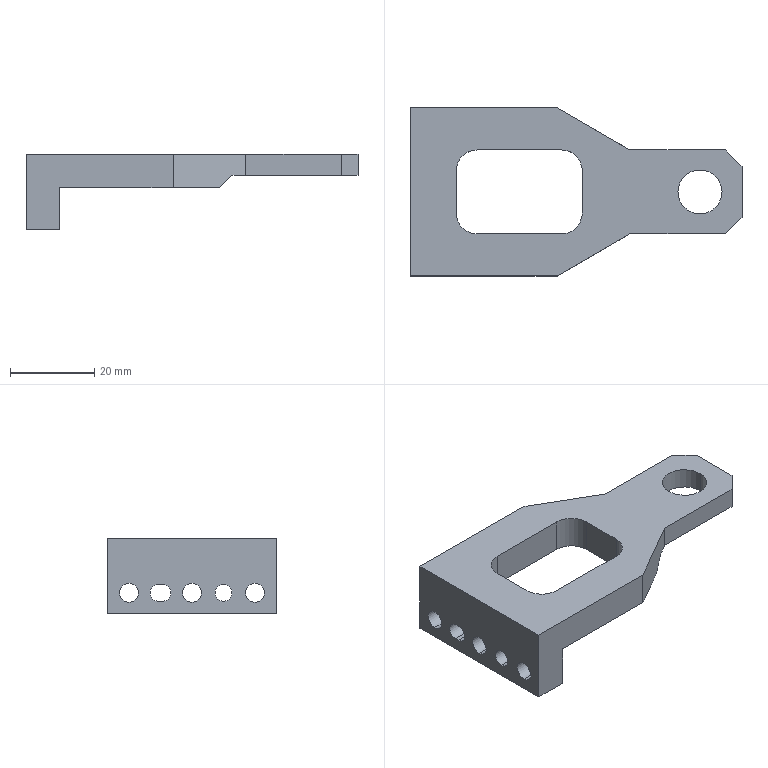Part | SolidWorks | features ICE 6, Chamfer 2, Extrusion 1, HoleWzd 1 | 1 solid | 38 faces | box 79 x 40 x 18 mm | volume 15138 mm3 | plane 22 | cylinder 16 | commonest cylinder face diameters 4.5 x6 4 x4 10 x4 10.5 x2
STEP:
#1=CARTESIAN_POINT('',(8.,12.5,5.601));
#2=VERTEX_POINT('',#1);
#3=CARTESIAN_POINT('',(8.,12.5,9.601));
#4=VERTEX_POINT('',#3);
#5=CARTESIAN_POINT('',(8.,12.5,7.601));
#6=DIRECTION('',(-1.,0.,0.));
#7=DIRECTION('',(0.,0.,1.));
#8=AXIS2_PLACEMENT_3D('',#5,#6,#7);
#9=CIRCLE('',#8,2.);
#10=EDGE_CURVE('',#2,#4,#9,.T.);
#11=ORIENTED_EDGE('',*,*,#10,.F.);
#12=CARTESIAN_POINT('',(0.,12.5,5.601));
#13=VERTEX_POINT('',#12);
#14=CARTESIAN_POINT('',(0.,12.5,5.601));
#15=DIRECTION('',(-1.,0.,0.));
#16=VECTOR('',#15,1000.);
#17=LINE('',#14,#16);
#18=EDGE_CURVE('',#2,#13,#17,.T.);
#19=ORIENTED_EDGE('',*,*,#18,.T.);
#20=CARTESIAN_POINT('',(0.,12.5,9.601));
#21=VERTEX_POINT('',#20);
#22=CARTESIAN_POINT('',(0.,12.5,7.601));
#23=DIRECTION('',(-1.,0.,0.));
#24=DIRECTION('',(0.,0.,1.));
#25=AXIS2_PLACEMENT_3D('',#22,#23,#24);
#26=CIRCLE('',#25,2.);
#27=EDGE_CURVE('',#13,#21,#26,.T.);
#28=ORIENTED_EDGE('',*,*,#27,.T.);
#29=CARTESIAN_POINT('',(0.,12.5,9.601));
#30=DIRECTION('',(-1.,0.,0.));
#31=VECTOR('',#30,1000.);
#32=LINE('',#29,#31);
#33=EDGE_CURVE('',#4,#21,#32,.T.);
#34=ORIENTED_EDGE('',*,*,#33,.F.);
#35=EDGE_LOOP('',(#11,#19,#28,#34));
#36=FACE_OUTER_BOUND('',#35,.T.);
#37=CARTESIAN_POINT('',(0.,12.5,7.601));
#38=DIRECTION('',(-1.,0.,0.));
#39=DIRECTION('',(0.,0.,1.));
#40=AXIS2_PLACEMENT_3D('',#37,#38,#39);
#41=CYLINDRICAL_SURFACE('',#40,2.);
#42=ADVANCED_FACE('',(#36),#41,.F.);
#43=CARTESIAN_POINT('',(0.,5.,9.851));
#44=VERTEX_POINT('',#43);
#45=CARTESIAN_POINT('',(0.,5.,5.351));
#46=VERTEX_POINT('',#45);
#47=CARTESIAN_POINT('',(0.,5.,7.601));
#48=DIRECTION('',(1.,0.,0.));
#49=DIRECTION('',(0.,0.,1.));
#50=AXIS2_PLACEMENT_3D('',#47,#48,#49);
#51=CIRCLE('',#50,2.25);
#52=EDGE_CURVE('',#44,#46,#51,.T.);
#53=ORIENTED_EDGE('',*,*,#52,.F.);
#54=CARTESIAN_POINT('',(8.,5.,9.851));
#55=VERTEX_POINT('',#54);
#56=CARTESIAN_POINT('',(0.,5.,9.851));
#57=DIRECTION('',(1.,0.,0.));
#58=VECTOR('',#57,1000.);
#59=LINE('',#56,#58);
#60=EDGE_CURVE('',#44,#55,#59,.T.);
#61=ORIENTED_EDGE('',*,*,#60,.T.);
#62=CARTESIAN_POINT('',(8.,5.,5.351));
#63=VERTEX_POINT('',#62);
#64=CARTESIAN_POINT('',(8.,5.,7.601));
#65=DIRECTION('',(1.,0.,0.));
#66=DIRECTION('',(0.,0.,1.));
#67=AXIS2_PLACEMENT_3D('',#64,#65,#66);
#68=CIRCLE('',#67,2.25);
#69=EDGE_CURVE('',#55,#63,#68,.T.);
#70=ORIENTED_EDGE('',*,*,#69,.T.);
#71=CARTESIAN_POINT('',(0.,5.,5.351));
#72=DIRECTION('',(1.,0.,0.));
#73=VECTOR('',#72,1000.);
#74=LINE('',#71,#73);
#75=EDGE_CURVE('',#46,#63,#74,.T.);
#76=ORIENTED_EDGE('',*,*,#75,.F.);
#77=EDGE_LOOP('',(#53,#61,#70,#76));
#78=FACE_OUTER_BOUND('',#77,.T.);
#79=CARTESIAN_POINT('',(0.,5.,7.601));
#80=DIRECTION('',(1.,0.,0.));
#81=DIRECTION('',(0.,0.,-1.));
#82=AXIS2_PLACEMENT_3D('',#79,#80,#81);
#83=CYLINDRICAL_SURFACE('',#82,2.25);
#84=ADVANCED_FACE('',(#78),#83,.F.);
#85=CARTESIAN_POINT('',(0.,20.,9.851));
#86=VERTEX_POINT('',#85);
#87=CARTESIAN_POINT('',(0.,20.,5.351));
#88=VERTEX_POINT('',#87);
#89=CARTESIAN_POINT('',(0.,20.,7.601));
#90=DIRECTION('',(1.,0.,0.));
#91=DIRECTION('',(0.,0.,-1.));
#92=AXIS2_PLACEMENT_3D('',#89,#90,#91);
#93=CIRCLE('',#92,2.25);
#94=EDGE_CURVE('',#86,#88,#93,.T.);
#95=ORIENTED_EDGE('',*,*,#94,.F.);
#96=CARTESIAN_POINT('',(8.,20.,9.851));
#97=VERTEX_POINT('',#96);
#98=CARTESIAN_POINT('',(0.,20.,9.851));
#99=DIRECTION('',(1.,0.,0.));
#100=VECTOR('',#99,1000.);
#101=LINE('',#98,#100);
#102=EDGE_CURVE('',#86,#97,#101,.T.);
#103=ORIENTED_EDGE('',*,*,#102,.T.);
#104=CARTESIAN_POINT('',(8.,20.,5.351));
#105=VERTEX_POINT('',#104);
#106=CARTESIAN_POINT('',(8.,20.,7.601));
#107=DIRECTION('',(1.,0.,0.));
#108=DIRECTION('',(0.,0.,-1.));
#109=AXIS2_PLACEMENT_3D('',#106,#107,#108);
#110=CIRCLE('',#109,2.25);
#111=EDGE_CURVE('',#97,#105,#110,.T.);
#112=ORIENTED_EDGE('',*,*,#111,.T.);
#113=CARTESIAN_POINT('',(0.,20.,5.351));
#114=DIRECTION('',(1.,0.,0.));
#115=VECTOR('',#114,1000.);
#116=LINE('',#113,#115);
#117=EDGE_CURVE('',#88,#105,#116,.T.);
#118=ORIENTED_EDGE('',*,*,#117,.F.);
#119=EDGE_LOOP('',(#95,#103,#112,#118));
#120=FACE_OUTER_BOUND('',#119,.T.);
#121=CARTESIAN_POINT('',(0.,20.,7.601));
#122=DIRECTION('',(1.,0.,0.));
#123=DIRECTION('',(0.,0.,-1.));
#124=AXIS2_PLACEMENT_3D('',#121,#122,#123);
#125=CYLINDRICAL_SURFACE('',#124,2.25);
#126=ADVANCED_FACE('',(#120),#125,.F.);
#127=CARTESIAN_POINT('',(0.,35.,9.851));
#128=VERTEX_POINT('',#127);
#129=CARTESIAN_POINT('',(0.,35.,5.351));
#130=VERTEX_POINT('',#129);
#131=CARTESIAN_POINT('',(0.,35.,7.601));
#132=DIRECTION('',(1.,0.,0.));
#133=DIRECTION('',(0.,0.,-1.));
#134=AXIS2_PLACEMENT_3D('',#131,#132,#133);
#135=CIRCLE('',#134,2.25);
#136=EDGE_CURVE('',#128,#130,#135,.T.);
#137=ORIENTED_EDGE('',*,*,#136,.F.);
#138=CARTESIAN_POINT('',(8.,35.,9.851));
#139=VERTEX_POINT('',#138);
#140=CARTESIAN_POINT('',(0.,35.,9.851));
#141=DIRECTION('',(1.,0.,0.));
#142=VECTOR('',#141,1000.);
#143=LINE('',#140,#142);
#144=EDGE_CURVE('',#128,#139,#143,.T.);
#145=ORIENTED_EDGE('',*,*,#144,.T.);
#146=CARTESIAN_POINT('',(8.,35.,5.351));
#147=VERTEX_POINT('',#146);
#148=CARTESIAN_POINT('',(8.,35.,7.601));
#149=DIRECTION('',(1.,0.,0.));
#150=DIRECTION('',(0.,0.,-1.));
#151=AXIS2_PLACEMENT_3D('',#148,#149,#150);
#152=CIRCLE('',#151,2.25);
#153=EDGE_CURVE('',#139,#147,#152,.T.);
#154=ORIENTED_EDGE('',*,*,#153,.T.);
#155=CARTESIAN_POINT('',(0.,35.,5.351));
#156=DIRECTION('',(1.,0.,0.));
#157=VECTOR('',#156,1000.);
#158=LINE('',#155,#157);
#159=EDGE_CURVE('',#130,#147,#158,.T.);
#160=ORIENTED_EDGE('',*,*,#159,.F.);
#161=EDGE_LOOP('',(#137,#145,#154,#160));
#162=FACE_OUTER_BOUND('',#161,.T.);
#163=CARTESIAN_POINT('',(0.,35.,7.601));
#164=DIRECTION('',(1.,0.,0.));
#165=DIRECTION('',(0.,0.,-1.));
#166=AXIS2_PLACEMENT_3D('',#163,#164,#165);
#167=CYLINDRICAL_SURFACE('',#166,2.25);
#168=ADVANCED_FACE('',(#162),#167,.F.);
#169=CARTESIAN_POINT('',(74.25,20.,20.601));
#170=VERTEX_POINT('',#169);
#171=CARTESIAN_POINT('',(63.75,20.,20.601));
#172=VERTEX_POINT('',#171);
#173=CARTESIAN_POINT('',(69.,20.,20.601));
#174=DIRECTION('',(0.,0.,-1.));
#175=DIRECTION('',(-1.,0.,0.));
#176=AXIS2_PLACEMENT_3D('',#173,#174,#175);
#177=CIRCLE('',#176,5.25);
#178=EDGE_CURVE('',#170,#172,#177,.T.);
#179=ORIENTED_EDGE('',*,*,#178,.F.);
#180=CARTESIAN_POINT('',(74.25,20.,15.601));
#181=VERTEX_POINT('',#180);
#182=CARTESIAN_POINT('',(74.25,20.,22.601));
#183=DIRECTION('',(0.,0.,-1.));
#184=VECTOR('',#183,1000.);
#185=LINE('',#182,#184);
#186=EDGE_CURVE('',#170,#181,#185,.T.);
#187=ORIENTED_EDGE('',*,*,#186,.T.);
#188=CARTESIAN_POINT('',(63.75,20.,15.601));
#189=VERTEX_POINT('',#188);
#190=CARTESIAN_POINT('',(69.,20.,15.601));
#191=DIRECTION('',(0.,0.,-1.));
#192=DIRECTION('',(1.,0.,0.));
#193=AXIS2_PLACEMENT_3D('',#190,#191,#192);
#194=CIRCLE('',#193,5.25);
#195=EDGE_CURVE('',#181,#189,#194,.T.);
#196=ORIENTED_EDGE('',*,*,#195,.T.);
#197=CARTESIAN_POINT('',(63.75,20.,22.601));
#198=DIRECTION('',(0.,0.,-1.));
#199=VECTOR('',#198,1000.);
#200=LINE('',#197,#199);
#201=EDGE_CURVE('',#172,#189,#200,.T.);
#202=ORIENTED_EDGE('',*,*,#201,.F.);
#203=EDGE_LOOP('',(#179,#187,#196,#202));
#204=FACE_OUTER_BOUND('',#203,.T.);
#205=CARTESIAN_POINT('',(69.,20.,22.601));
#206=DIRECTION('',(0.,0.,-1.));
#207=DIRECTION('',(-1.,0.,0.));
#208=AXIS2_PLACEMENT_3D('',#205,#206,#207);
#209=CYLINDRICAL_SURFACE('',#208,5.25);
#210=ADVANCED_FACE('',(#204),#209,.F.);
#211=CARTESIAN_POINT('',(8.,27.,9.601));
#212=VERTEX_POINT('',#211);
#213=CARTESIAN_POINT('',(8.,28.,9.601));
#214=VERTEX_POINT('',#213);
#215=CARTESIAN_POINT('',(8.,40.,9.601));
#216=DIRECTION('',(0.,1.,0.));
#217=VECTOR('',#216,1000.);
#218=LINE('',#215,#217);
#219=EDGE_CURVE('',#212,#214,#218,.T.);
#220=ORIENTED_EDGE('',*,*,#219,.T.);
#221=CARTESIAN_POINT('',(8.,28.,5.601));
#222=VERTEX_POINT('',#221);
#223=CARTESIAN_POINT('',(8.,28.,7.601));
#224=DIRECTION('',(-1.,0.,0.));
#225=DIRECTION('',(0.,0.,1.));
#226=AXIS2_PLACEMENT_3D('',#223,#224,#225);
#227=CIRCLE('',#226,2.);
#228=EDGE_CURVE('',#214,#222,#227,.T.);
#229=ORIENTED_EDGE('',*,*,#228,.T.);
#230=CARTESIAN_POINT('',(8.,27.,5.601));
#231=VERTEX_POINT('',#230);
#232=CARTESIAN_POINT('',(8.,40.,5.601));
#233=DIRECTION('',(0.,-1.,0.));
#234=VECTOR('',#233,1000.);
#235=LINE('',#232,#234);
#236=EDGE_CURVE('',#222,#231,#235,.T.);
#237=ORIENTED_EDGE('',*,*,#236,.T.);
#238=CARTESIAN_POINT('',(8.,27.,7.601));
#239=DIRECTION('',(-1.,0.,0.));
#240=DIRECTION('',(0.,0.,1.));
#241=AXIS2_PLACEMENT_3D('',#238,#239,#240);
#242=CIRCLE('',#241,2.);
#243=EDGE_CURVE('',#231,#212,#242,.T.);
#244=ORIENTED_EDGE('',*,*,#243,.T.);
#245=EDGE_LOOP('',(#220,#229,#237,#244));
#246=FACE_BOUND('',#245,.T.);
#247=CARTESIAN_POINT('',(8.,12.5,7.601));
#248=DIRECTION('',(-1.,0.,0.));
#249=DIRECTION('',(0.,0.,1.));
#250=AXIS2_PLACEMENT_3D('',#247,#248,#249);
#251=CIRCLE('',#250,2.);
#252=EDGE_CURVE('',#4,#2,#251,.T.);
#253=ORIENTED_EDGE('',*,*,#252,.T.);
#254=ORIENTED_EDGE('',*,*,#10,.T.);
#255=EDGE_LOOP('',(#253,#254));
#256=FACE_BOUND('',#255,.T.);
#257=CARTESIAN_POINT('',(8.,5.,7.601));
#258=DIRECTION('',(1.,0.,0.));
#259=DIRECTION('',(0.,0.,1.));
#260=AXIS2_PLACEMENT_3D('',#257,#258,#259);
#261=CIRCLE('',#260,2.25);
#262=EDGE_CURVE('',#63,#55,#261,.T.);
#263=ORIENTED_EDGE('',*,*,#262,.F.);
#264=ORIENTED_EDGE('',*,*,#69,.F.);
#265=EDGE_LOOP('',(#263,#264));
#266=FACE_BOUND('',#265,.T.);
#267=CARTESIAN_POINT('',(8.,20.,7.601));
#268=DIRECTION('',(1.,0.,0.));
#269=DIRECTION('',(0.,0.,-1.));
#270=AXIS2_PLACEMENT_3D('',#267,#268,#269);
#271=CIRCLE('',#270,2.25);
#272=EDGE_CURVE('',#105,#97,#271,.T.);
#273=ORIENTED_EDGE('',*,*,#272,.F.);
#274=ORIENTED_EDGE('',*,*,#111,.F.);
#275=EDGE_LOOP('',(#273,#274));
#276=FACE_BOUND('',#275,.T.);
#277=CARTESIAN_POINT('',(8.,35.,7.601));
#278=DIRECTION('',(1.,0.,0.));
#279=DIRECTION('',(0.,0.,-1.));
#280=AXIS2_PLACEMENT_3D('',#277,#278,#279);
#281=CIRCLE('',#280,2.25);
#282=EDGE_CURVE('',#147,#139,#281,.T.);
#283=ORIENTED_EDGE('',*,*,#282,.F.);
#284=ORIENTED_EDGE('',*,*,#153,.F.);
#285=EDGE_LOOP('',(#283,#284));
#286=FACE_BOUND('',#285,.T.);
#287=CARTESIAN_POINT('',(8.,0.,12.601));
#288=VERTEX_POINT('',#287);
#289=CARTESIAN_POINT('',(8.,0.,2.601));
#290=VERTEX_POINT('',#289);
#291=CARTESIAN_POINT('',(8.,0.,12.601));
#292=DIRECTION('',(0.,0.,-1.));
#293=VECTOR('',#292,1000.);
#294=LINE('',#291,#293);
#295=EDGE_CURVE('',#288,#290,#294,.T.);
#296=ORIENTED_EDGE('',*,*,#295,.T.);
#297=CARTESIAN_POINT('',(8.,40.,2.601));
#298=VERTEX_POINT('',#297);
#299=CARTESIAN_POINT('',(8.,40.,2.601));
#300=DIRECTION('',(0.,-1.,0.));
#301=VECTOR('',#300,1000.);
#302=LINE('',#299,#301);
#303=EDGE_CURVE('',#298,#290,#302,.T.);
#304=ORIENTED_EDGE('',*,*,#303,.F.);
#305=CARTESIAN_POINT('',(8.,40.,12.601));
#306=VERTEX_POINT('',#305);
#307=CARTESIAN_POINT('',(8.,40.,12.601));
#308=DIRECTION('',(0.,0.,-1.));
#309=VECTOR('',#308,1000.);
#310=LINE('',#307,#309);
#311=EDGE_CURVE('',#306,#298,#310,.T.);
#312=ORIENTED_EDGE('',*,*,#311,.F.);
#313=CARTESIAN_POINT('',(8.,40.,12.601));
#314=DIRECTION('',(0.,-1.,0.));
#315=VECTOR('',#314,1000.);
#316=LINE('',#313,#315);
#317=EDGE_CURVE('',#306,#288,#316,.T.);
#318=ORIENTED_EDGE('',*,*,#317,.T.);
#319=EDGE_LOOP('',(#296,#304,#312,#318));
#320=FACE_OUTER_BOUND('',#319,.T.);
#321=CARTESIAN_POINT('',(8.,40.,12.601));
#322=DIRECTION('',(-1.,0.,0.));
#323=DIRECTION('',(0.,0.,1.));
#324=AXIS2_PLACEMENT_3D('',#321,#322,#323);
#325=PLANE('',#324);
#326=ADVANCED_FACE('',(#246,#256,#266,#276,#286,#320),#325,.F.);
#327=CARTESIAN_POINT('',(0.,0.,2.601));
#328=VERTEX_POINT('',#327);
#329=CARTESIAN_POINT('',(0.,0.,2.601));
#330=DIRECTION('',(-1.,0.,0.));
#331=VECTOR('',#330,1000.);
#332=LINE('',#329,#331);
#333=EDGE_CURVE('',#290,#328,#332,.T.);
#334=ORIENTED_EDGE('',*,*,#333,.T.);
#335=CARTESIAN_POINT('',(0.,40.,2.601));
#336=VERTEX_POINT('',#335);
#337=CARTESIAN_POINT('',(0.,40.,2.601));
#338=DIRECTION('',(0.,-1.,0.));
#339=VECTOR('',#338,1000.);
#340=LINE('',#337,#339);
#341=EDGE_CURVE('',#336,#328,#340,.T.);
#342=ORIENTED_EDGE('',*,*,#341,.F.);
#343=CARTESIAN_POINT('',(0.,40.,2.601));
#344=DIRECTION('',(-1.,0.,0.));
#345=VECTOR('',#344,1000.);
#346=LINE('',#343,#345);
#347=EDGE_CURVE('',#298,#336,#346,.T.);
#348=ORIENTED_EDGE('',*,*,#347,.F.);
#349=ORIENTED_EDGE('',*,*,#303,.T.);
#350=EDGE_LOOP('',(#334,#342,#348,#349));
#351=FACE_OUTER_BOUND('',#350,.T.);
#352=CARTESIAN_POINT('',(0.,40.,2.601));
#353=DIRECTION('',(0.,0.,1.));
#354=DIRECTION('',(1.,0.,0.));
#355=AXIS2_PLACEMENT_3D('',#352,#353,#354);
#356=PLANE('',#355);
#357=ADVANCED_FACE('',(#351),#356,.F.);
#358=CARTESIAN_POINT('',(0.,28.,5.601));
#359=VERTEX_POINT('',#358);
#360=CARTESIAN_POINT('',(0.,27.,5.601));
#361=VERTEX_POINT('',#360);
#362=CARTESIAN_POINT('',(0.,28.,5.601));
#363=DIRECTION('',(0.,-1.,0.));
#364=VECTOR('',#363,1000.);
#365=LINE('',#362,#364);
#366=EDGE_CURVE('',#359,#361,#365,.T.);
#367=ORIENTED_EDGE('',*,*,#366,.F.);
#368=CARTESIAN_POINT('',(0.,28.,9.601));
#369=VERTEX_POINT('',#368);
#370=CARTESIAN_POINT('',(0.,28.,7.601));
#371=DIRECTION('',(-1.,0.,0.));
#372=DIRECTION('',(0.,0.,1.));
#373=AXIS2_PLACEMENT_3D('',#370,#371,#372);
#374=CIRCLE('',#373,2.);
#375=EDGE_CURVE('',#369,#359,#374,.T.);
#376=ORIENTED_EDGE('',*,*,#375,.F.);
#377=CARTESIAN_POINT('',(0.,27.,9.601));
#378=VERTEX_POINT('',#377);
#379=CARTESIAN_POINT('',(0.,28.,9.601));
#380=DIRECTION('',(0.,1.,0.));
#381=VECTOR('',#380,1000.);
#382=LINE('',#379,#381);
#383=EDGE_CURVE('',#378,#369,#382,.T.);
#384=ORIENTED_EDGE('',*,*,#383,.F.);
#385=CARTESIAN_POINT('',(0.,27.,7.601));
#386=DIRECTION('',(-1.,0.,0.));
#387=DIRECTION('',(0.,0.,1.));
#388=AXIS2_PLACEMENT_3D('',#385,#386,#387);
#389=CIRCLE('',#388,2.);
#390=EDGE_CURVE('',#361,#378,#389,.T.);
#391=ORIENTED_EDGE('',*,*,#390,.F.);
#392=EDGE_LOOP('',(#367,#376,#384,#391));
#393=FACE_BOUND('',#392,.T.);
#394=CARTESIAN_POINT('',(0.,12.5,7.601));
#395=DIRECTION('',(-1.,0.,0.));
#396=DIRECTION('',(0.,0.,1.));
#397=AXIS2_PLACEMENT_3D('',#394,#395,#396);
#398=CIRCLE('',#397,2.);
#399=EDGE_CURVE('',#21,#13,#398,.T.);
#400=ORIENTED_EDGE('',*,*,#399,.F.);
#401=ORIENTED_EDGE('',*,*,#27,.F.);
#402=EDGE_LOOP('',(#400,#401));
#403=FACE_BOUND('',#402,.T.);
#404=CARTESIAN_POINT('',(0.,5.,7.601));
#405=DIRECTION('',(1.,0.,0.));
#406=DIRECTION('',(0.,0.,1.));
#407=AXIS2_PLACEMENT_3D('',#404,#405,#406);
#408=CIRCLE('',#407,2.25);
#409=EDGE_CURVE('',#46,#44,#408,.T.);
#410=ORIENTED_EDGE('',*,*,#409,.T.);
#411=ORIENTED_EDGE('',*,*,#52,.T.);
#412=EDGE_LOOP('',(#410,#411));
#413=FACE_BOUND('',#412,.T.);
#414=CARTESIAN_POINT('',(0.,20.,7.601));
#415=DIRECTION('',(1.,0.,0.));
#416=DIRECTION('',(0.,0.,-1.));
#417=AXIS2_PLACEMENT_3D('',#414,#415,#416);
#418=CIRCLE('',#417,2.25);
#419=EDGE_CURVE('',#88,#86,#418,.T.);
#420=ORIENTED_EDGE('',*,*,#419,.T.);
#421=ORIENTED_EDGE('',*,*,#94,.T.);
#422=EDGE_LOOP('',(#420,#421));
#423=FACE_BOUND('',#422,.T.);
#424=CARTESIAN_POINT('',(0.,35.,7.601));
#425=DIRECTION('',(1.,0.,0.));
#426=DIRECTION('',(0.,0.,-1.));
#427=AXIS2_PLACEMENT_3D('',#424,#425,#426);
#428=CIRCLE('',#427,2.25);
#429=EDGE_CURVE('',#130,#128,#428,.T.);
#430=ORIENTED_EDGE('',*,*,#429,.T.);
#431=ORIENTED_EDGE('',*,*,#136,.T.);
#432=EDGE_LOOP('',(#430,#431));
#433=FACE_BOUND('',#432,.T.);
#434=CARTESIAN_POINT('',(0.,0.,20.601));
#435=VERTEX_POINT('',#434);
#436=CARTESIAN_POINT('',(0.,0.,20.601));
#437=DIRECTION('',(0.,0.,1.));
#438=VECTOR('',#437,1000.);
#439=LINE('',#436,#438);
#440=EDGE_CURVE('',#328,#435,#439,.T.);
#441=ORIENTED_EDGE('',*,*,#440,.T.);
#442=CARTESIAN_POINT('',(0.,40.,20.601));
#443=VERTEX_POINT('',#442);
#444=CARTESIAN_POINT('',(0.,40.,20.601));
#445=DIRECTION('',(0.,-1.,0.));
#446=VECTOR('',#445,1000.);
#447=LINE('',#444,#446);
#448=EDGE_CURVE('',#443,#435,#447,.T.);
#449=ORIENTED_EDGE('',*,*,#448,.F.);
#450=CARTESIAN_POINT('',(0.,40.,20.601));
#451=DIRECTION('',(0.,0.,1.));
#452=VECTOR('',#451,1000.);
#453=LINE('',#450,#452);
#454=EDGE_CURVE('',#336,#443,#453,.T.);
#455=ORIENTED_EDGE('',*,*,#454,.F.);
#456=ORIENTED_EDGE('',*,*,#341,.T.);
#457=EDGE_LOOP('',(#441,#449,#455,#456));
#458=FACE_OUTER_BOUND('',#457,.T.);
#459=CARTESIAN_POINT('',(0.,40.,20.601));
#460=DIRECTION('',(1.,0.,0.));
#461=DIRECTION('',(0.,0.,-1.));
#462=AXIS2_PLACEMENT_3D('',#459,#460,#461);
#463=PLANE('',#462);
#464=ADVANCED_FACE('',(#393,#403,#413,#423,#433,#458),#463,.F.);
#465=CARTESIAN_POINT('',(11.,25.,20.601));
#466=VERTEX_POINT('',#465);
#467=CARTESIAN_POINT('',(11.,15.,20.601));
#468=VERTEX_POINT('',#467);
#469=CARTESIAN_POINT('',(11.,15.,20.601));
#470=DIRECTION('',(0.,-1.,0.));
#471=VECTOR('',#470,1000.);
#472=LINE('',#469,#471);
#473=EDGE_CURVE('',#466,#468,#472,.T.);
#474=ORIENTED_EDGE('',*,*,#473,.F.);
#475=CARTESIAN_POINT('',(16.,30.,20.601));
#476=VERTEX_POINT('',#475);
#477=CARTESIAN_POINT('',(16.,25.,20.601));
#478=DIRECTION('',(0.,0.,1.));
#479=DIRECTION('',(1.,0.,0.));
#480=AXIS2_PLACEMENT_3D('',#477,#478,#479);
#481=CIRCLE('',#480,5.);
#482=EDGE_CURVE('',#476,#466,#481,.T.);
#483=ORIENTED_EDGE('',*,*,#482,.F.);
#484=CARTESIAN_POINT('',(36.,30.,20.601));
#485=VERTEX_POINT('',#484);
#486=CARTESIAN_POINT('',(16.,30.,20.601));
#487=DIRECTION('',(-1.,0.,0.));
#488=VECTOR('',#487,1000.);
#489=LINE('',#486,#488);
#490=EDGE_CURVE('',#485,#476,#489,.T.);
#491=ORIENTED_EDGE('',*,*,#490,.F.);
#492=CARTESIAN_POINT('',(41.,25.,20.601));
#493=VERTEX_POINT('',#492);
#494=CARTESIAN_POINT('',(36.,25.,20.601));
#495=DIRECTION('',(0.,0.,1.));
#496=DIRECTION('',(1.,0.,0.));
#497=AXIS2_PLACEMENT_3D('',#494,#495,#496);
#498=CIRCLE('',#497,5.);
#499=EDGE_CURVE('',#493,#485,#498,.T.);
#500=ORIENTED_EDGE('',*,*,#499,.F.);
#501=CARTESIAN_POINT('',(41.,15.,20.601));
#502=VERTEX_POINT('',#501);
#503=CARTESIAN_POINT('',(41.,15.,20.601));
#504=DIRECTION('',(0.,1.,0.));
#505=VECTOR('',#504,1000.);
#506=LINE('',#503,#505);
#507=EDGE_CURVE('',#502,#493,#506,.T.);
#508=ORIENTED_EDGE('',*,*,#507,.F.);
#509=CARTESIAN_POINT('',(36.,10.,20.601));
#510=VERTEX_POINT('',#509);
#511=CARTESIAN_POINT('',(36.,15.,20.601));
#512=DIRECTION('',(0.,0.,1.));
#513=DIRECTION('',(1.,0.,0.));
#514=AXIS2_PLACEMENT_3D('',#511,#512,#513);
#515=CIRCLE('',#514,5.);
#516=EDGE_CURVE('',#510,#502,#515,.T.);
#517=ORIENTED_EDGE('',*,*,#516,.F.);
#518=CARTESIAN_POINT('',(16.,10.,20.601));
#519=VERTEX_POINT('',#518);
#520=CARTESIAN_POINT('',(16.,10.,20.601));
#521=DIRECTION('',(1.,0.,0.));
#522=VECTOR('',#521,1000.);
#523=LINE('',#520,#522);
#524=EDGE_CURVE('',#519,#510,#523,.T.);
#525=ORIENTED_EDGE('',*,*,#524,.F.);
#526=CARTESIAN_POINT('',(16.,15.,20.601));
#527=DIRECTION('',(0.,0.,1.));
#528=DIRECTION('',(1.,0.,0.));
#529=AXIS2_PLACEMENT_3D('',#526,#527,#528);
#530=CIRCLE('',#529,5.);
#531=EDGE_CURVE('',#468,#519,#530,.T.);
#532=ORIENTED_EDGE('',*,*,#531,.F.);
#533=EDGE_LOOP('',(#474,#483,#491,#500,#508,#517,#525,#532));
#534=FACE_BOUND('',#533,.T.);
#535=CARTESIAN_POINT('',(69.,20.,20.601));
#536=DIRECTION('',(0.,0.,-1.));
#537=DIRECTION('',(-1.,0.,0.));
#538=AXIS2_PLACEMENT_3D('',#535,#536,#537);
#539=CIRCLE('',#538,5.25);
#540=EDGE_CURVE('',#172,#170,#539,.T.);
#541=ORIENTED_EDGE('',*,*,#540,.T.);
#542=ORIENTED_EDGE('',*,*,#178,.T.);
#543=EDGE_LOOP('',(#541,#542));
#544=FACE_BOUND('',#543,.T.);
#545=CARTESIAN_POINT('',(75.,10.,20.601));
#546=VERTEX_POINT('',#545);
#547=CARTESIAN_POINT('',(52.321,10.,20.601));
#548=VERTEX_POINT('',#547);
#549=CARTESIAN_POINT('',(79.,10.,20.601));
#550=DIRECTION('',(-1.,0.,0.));
#551=VECTOR('',#550,1000.);
#552=LINE('',#549,#551);
#553=EDGE_CURVE('',#546,#548,#552,.T.);
#554=ORIENTED_EDGE('',*,*,#553,.F.);
#555=CARTESIAN_POINT('',(79.,14.,20.601));
#556=VERTEX_POINT('',#555);
#557=CARTESIAN_POINT('',(75.,10.,20.601));
#558=DIRECTION('',(0.7071,0.7071,0.));
#559=VECTOR('',#558,1000.);
#560=LINE('',#557,#559);
#561=EDGE_CURVE('',#546,#556,#560,.T.);
#562=ORIENTED_EDGE('',*,*,#561,.T.);
#563=CARTESIAN_POINT('',(79.,26.,20.601));
#564=VERTEX_POINT('',#563);
#565=CARTESIAN_POINT('',(79.,40.,20.601));
#566=DIRECTION('',(0.,-1.,0.));
#567=VECTOR('',#566,1000.);
#568=LINE('',#565,#567);
#569=EDGE_CURVE('',#564,#556,#568,.T.);
#570=ORIENTED_EDGE('',*,*,#569,.F.);
#571=CARTESIAN_POINT('',(75.,30.,20.601));
#572=VERTEX_POINT('',#571);
#573=CARTESIAN_POINT('',(79.,26.,20.601));
#574=DIRECTION('',(-0.7071,0.7071,0.));
#575=VECTOR('',#574,1000.);
#576=LINE('',#573,#575);
#577=EDGE_CURVE('',#564,#572,#576,.T.);
#578=ORIENTED_EDGE('',*,*,#577,.T.);
#579=CARTESIAN_POINT('',(52.321,30.,20.601));
#580=VERTEX_POINT('',#579);
#581=CARTESIAN_POINT('',(79.,30.,20.601));
#582=DIRECTION('',(1.,0.,0.));
#583=VECTOR('',#582,1000.);
#584=LINE('',#581,#583);
#585=EDGE_CURVE('',#580,#572,#584,.T.);
#586=ORIENTED_EDGE('',*,*,#585,.F.);
#587=CARTESIAN_POINT('',(35.,40.,20.601));
#588=VERTEX_POINT('',#587);
#589=CARTESIAN_POINT('',(35.,40.,20.601));
#590=DIRECTION('',(0.866,-0.5,0.));
#591=VECTOR('',#590,1000.);
#592=LINE('',#589,#591);
#593=EDGE_CURVE('',#588,#580,#592,.T.);
#594=ORIENTED_EDGE('',*,*,#593,.F.);
#595=CARTESIAN_POINT('',(0.,40.,20.601));
#596=DIRECTION('',(1.,0.,0.));
#597=VECTOR('',#596,1000.);
#598=LINE('',#595,#597);
#599=EDGE_CURVE('',#443,#588,#598,.T.);
#600=ORIENTED_EDGE('',*,*,#599,.F.);
#601=ORIENTED_EDGE('',*,*,#448,.T.);
#602=CARTESIAN_POINT('',(35.,0.,20.601));
#603=VERTEX_POINT('',#602);
#604=CARTESIAN_POINT('',(0.,0.,20.601));
#605=DIRECTION('',(1.,0.,0.));
#606=VECTOR('',#605,1000.);
#607=LINE('',#604,#606);
#608=EDGE_CURVE('',#435,#603,#607,.T.);
#609=ORIENTED_EDGE('',*,*,#608,.T.);
#610=CARTESIAN_POINT('',(35.,0.,20.601));
#611=DIRECTION('',(-0.866,-0.5,0.));
#612=VECTOR('',#611,1000.);
#613=LINE('',#610,#612);
#614=EDGE_CURVE('',#548,#603,#613,.T.);
#615=ORIENTED_EDGE('',*,*,#614,.F.);
#616=EDGE_LOOP('',(#554,#562,#570,#578,#586,#594,#600,#601,#609,#615));
#617=FACE_OUTER_BOUND('',#616,.T.);
#618=CARTESIAN_POINT('',(0.,40.,20.601));
#619=DIRECTION('',(0.,0.,-1.));
#620=DIRECTION('',(-1.,0.,0.));
#621=AXIS2_PLACEMENT_3D('',#618,#619,#620);
#622=PLANE('',#621);
#623=ADVANCED_FACE('',(#534,#544,#617),#622,.F.);
#624=ORIENTED_EDGE('',*,*,#569,.T.);
#625=CARTESIAN_POINT('',(79.,14.,15.601));
#626=VERTEX_POINT('',#625);
#627=CARTESIAN_POINT('',(79.,14.,20.601));
#628=DIRECTION('',(0.,0.,-1.));
#629=VECTOR('',#628,1000.);
#630=LINE('',#627,#629);
#631=EDGE_CURVE('',#556,#626,#630,.T.);
#632=ORIENTED_EDGE('',*,*,#631,.T.);
#633=CARTESIAN_POINT('',(79.,26.,15.601));
#634=VERTEX_POINT('',#633);
#635=CARTESIAN_POINT('',(79.,0.,15.601));
#636=DIRECTION('',(0.,1.,0.));
#637=VECTOR('',#636,1000.);
#638=LINE('',#635,#637);
#639=EDGE_CURVE('',#626,#634,#638,.T.);
#640=ORIENTED_EDGE('',*,*,#639,.T.);
#641=CARTESIAN_POINT('',(79.,26.,20.601));
#642=DIRECTION('',(0.,0.,1.));
#643=VECTOR('',#642,1000.);
#644=LINE('',#641,#643);
#645=EDGE_CURVE('',#634,#564,#644,.T.);
#646=ORIENTED_EDGE('',*,*,#645,.T.);
#647=EDGE_LOOP('',(#624,#632,#640,#646));
#648=FACE_OUTER_BOUND('',#647,.T.);
#649=CARTESIAN_POINT('',(79.,40.,20.601));
#650=DIRECTION('',(-1.,0.,0.));
#651=DIRECTION('',(0.,0.,1.));
#652=AXIS2_PLACEMENT_3D('',#649,#650,#651);
#653=PLANE('',#652);
#654=ADVANCED_FACE('',(#648),#653,.F.);
#655=CARTESIAN_POINT('',(36.,30.,12.601));
#656=VERTEX_POINT('',#655);
#657=CARTESIAN_POINT('',(16.,30.,12.601));
#658=VERTEX_POINT('',#657);
#659=CARTESIAN_POINT('',(79.,30.,12.601));
#660=DIRECTION('',(-1.,0.,0.));
#661=VECTOR('',#660,1000.);
#662=LINE('',#659,#661);
#663=EDGE_CURVE('',#656,#658,#662,.T.);
#664=ORIENTED_EDGE('',*,*,#663,.T.);
#665=CARTESIAN_POINT('',(11.,25.,12.601));
#666=VERTEX_POINT('',#665);
#667=CARTESIAN_POINT('',(16.,25.,12.601));
#668=DIRECTION('',(0.,0.,1.));
#669=DIRECTION('',(1.,0.,0.));
#670=AXIS2_PLACEMENT_3D('',#667,#668,#669);
#671=CIRCLE('',#670,5.);
#672=EDGE_CURVE('',#658,#666,#671,.T.);
#673=ORIENTED_EDGE('',*,*,#672,.T.);
#674=CARTESIAN_POINT('',(11.,15.,12.601));
#675=VERTEX_POINT('',#674);
#676=CARTESIAN_POINT('',(11.,40.,12.601));
#677=DIRECTION('',(0.,-1.,0.));
#678=VECTOR('',#677,1000.);
#679=LINE('',#676,#678);
#680=EDGE_CURVE('',#666,#675,#679,.T.);
#681=ORIENTED_EDGE('',*,*,#680,.T.);
#682=CARTESIAN_POINT('',(16.,10.,12.601));
#683=VERTEX_POINT('',#682);
#684=CARTESIAN_POINT('',(16.,15.,12.601));
#685=DIRECTION('',(0.,0.,1.));
#686=DIRECTION('',(1.,0.,0.));
#687=AXIS2_PLACEMENT_3D('',#684,#685,#686);
#688=CIRCLE('',#687,5.);
#689=EDGE_CURVE('',#675,#683,#688,.T.);
#690=ORIENTED_EDGE('',*,*,#689,.T.);
#691=CARTESIAN_POINT('',(36.,10.,12.601));
#692=VERTEX_POINT('',#691);
#693=CARTESIAN_POINT('',(79.,10.,12.601));
#694=DIRECTION('',(1.,0.,0.));
#695=VECTOR('',#694,1000.);
#696=LINE('',#693,#695);
#697=EDGE_CURVE('',#683,#692,#696,.T.);
#698=ORIENTED_EDGE('',*,*,#697,.T.);
#699=CARTESIAN_POINT('',(41.,15.,12.601));
#700=VERTEX_POINT('',#699);
#701=CARTESIAN_POINT('',(36.,15.,12.601));
#702=DIRECTION('',(0.,0.,1.));
#703=DIRECTION('',(1.,0.,0.));
#704=AXIS2_PLACEMENT_3D('',#701,#702,#703);
#705=CIRCLE('',#704,5.);
#706=EDGE_CURVE('',#692,#700,#705,.T.);
#707=ORIENTED_EDGE('',*,*,#706,.T.);
#708=CARTESIAN_POINT('',(41.,25.,12.601));
#709=VERTEX_POINT('',#708);
#710=CARTESIAN_POINT('',(41.,40.,12.601));
#711=DIRECTION('',(0.,1.,0.));
#712=VECTOR('',#711,1000.);
#713=LINE('',#710,#712);
#714=EDGE_CURVE('',#700,#709,#713,.T.);
#715=ORIENTED_EDGE('',*,*,#714,.T.);
#716=CARTESIAN_POINT('',(36.,25.,12.601));
#717=DIRECTION('',(0.,0.,1.));
#718=DIRECTION('',(1.,0.,0.));
#719=AXIS2_PLACEMENT_3D('',#716,#717,#718);
#720=CIRCLE('',#719,5.);
#721=EDGE_CURVE('',#709,#656,#720,.T.);
#722=ORIENTED_EDGE('',*,*,#721,.T.);
#723=EDGE_LOOP('',(#664,#673,#681,#690,#698,#707,#715,#722));
#724=FACE_BOUND('',#723,.T.);
#725=CARTESIAN_POINT('',(35.,40.,12.601));
#726=VERTEX_POINT('',#725);
#727=CARTESIAN_POINT('',(46.,33.649,12.601));
#728=VERTEX_POINT('',#727);
#729=CARTESIAN_POINT('',(68.,20.947,12.601));
#730=DIRECTION('',(0.866,-0.5,0.));
#731=VECTOR('',#730,1000.);
#732=LINE('',#729,#731);
#733=EDGE_CURVE('',#726,#728,#732,.T.);
#734=ORIENTED_EDGE('',*,*,#733,.T.);
#735=CARTESIAN_POINT('',(46.,6.351,12.601));
#736=VERTEX_POINT('',#735);
#737=CARTESIAN_POINT('',(46.,40.,12.601));
#738=DIRECTION('',(0.,-1.,0.));
#739=VECTOR('',#738,1000.);
#740=LINE('',#737,#739);
#741=EDGE_CURVE('',#728,#736,#740,.T.);
#742=ORIENTED_EDGE('',*,*,#741,.T.);
#743=CARTESIAN_POINT('',(35.,0.,12.601));
#744=VERTEX_POINT('',#743);
#745=CARTESIAN_POINT('',(85.321,29.053,12.601));
#746=DIRECTION('',(-0.866,-0.5,0.));
#747=VECTOR('',#746,1000.);
#748=LINE('',#745,#747);
#749=EDGE_CURVE('',#736,#744,#748,.T.);
#750=ORIENTED_EDGE('',*,*,#749,.T.);
#751=CARTESIAN_POINT('',(79.,0.,12.601));
#752=DIRECTION('',(-1.,0.,0.));
#753=VECTOR('',#752,1000.);
#754=LINE('',#751,#753);
#755=EDGE_CURVE('',#744,#288,#754,.T.);
#756=ORIENTED_EDGE('',*,*,#755,.T.);
#757=ORIENTED_EDGE('',*,*,#317,.F.);
#758=CARTESIAN_POINT('',(79.,40.,12.601));
#759=DIRECTION('',(-1.,0.,0.));
#760=VECTOR('',#759,1000.);
#761=LINE('',#758,#760);
#762=EDGE_CURVE('',#726,#306,#761,.T.);
#763=ORIENTED_EDGE('',*,*,#762,.F.);
#764=EDGE_LOOP('',(#734,#742,#750,#756,#757,#763));
#765=FACE_OUTER_BOUND('',#764,.T.);
#766=CARTESIAN_POINT('',(79.,40.,12.601));
#767=DIRECTION('',(0.,0.,1.));
#768=DIRECTION('',(1.,0.,0.));
#769=AXIS2_PLACEMENT_3D('',#766,#767,#768);
#770=PLANE('',#769);
#771=ADVANCED_FACE('',(#724,#765),#770,.F.);
#772=ORIENTED_EDGE('',*,*,#599,.T.);
#773=CARTESIAN_POINT('',(35.,40.,0.));
#774=DIRECTION('',(0.,0.,-1.));
#775=VECTOR('',#774,1000.);
#776=LINE('',#773,#775);
#777=EDGE_CURVE('',#588,#726,#776,.T.);
#778=ORIENTED_EDGE('',*,*,#777,.T.);
#779=ORIENTED_EDGE('',*,*,#762,.T.);
#780=ORIENTED_EDGE('',*,*,#311,.T.);
#781=ORIENTED_EDGE('',*,*,#347,.T.);
#782=ORIENTED_EDGE('',*,*,#454,.T.);
#783=EDGE_LOOP('',(#772,#778,#779,#780,#781,#782));
#784=FACE_OUTER_BOUND('',#783,.T.);
#785=CARTESIAN_POINT('',(0.,40.,0.));
#786=DIRECTION('',(0.,-1.,0.));
#787=DIRECTION('',(0.,0.,-1.));
#788=AXIS2_PLACEMENT_3D('',#785,#786,#787);
#789=PLANE('',#788);
#790=ADVANCED_FACE('',(#784),#789,.F.);
#791=CARTESIAN_POINT('',(35.,0.,0.));
#792=DIRECTION('',(0.,0.,-1.));
#793=VECTOR('',#792,1000.);
#794=LINE('',#791,#793);
#795=EDGE_CURVE('',#603,#744,#794,.T.);
#796=ORIENTED_EDGE('',*,*,#795,.F.);
#797=ORIENTED_EDGE('',*,*,#608,.F.);
#798=ORIENTED_EDGE('',*,*,#440,.F.);
#799=ORIENTED_EDGE('',*,*,#333,.F.);
#800=ORIENTED_EDGE('',*,*,#295,.F.);
#801=ORIENTED_EDGE('',*,*,#755,.F.);
#802=EDGE_LOOP('',(#796,#797,#798,#799,#800,#801));
#803=FACE_OUTER_BOUND('',#802,.T.);
#804=CARTESIAN_POINT('',(0.,0.,0.));
#805=DIRECTION('',(0.,-1.,0.));
#806=DIRECTION('',(0.,0.,-1.));
#807=AXIS2_PLACEMENT_3D('',#804,#805,#806);
#808=PLANE('',#807);
#809=ADVANCED_FACE('',(#803),#808,.T.);
#810=ORIENTED_EDGE('',*,*,#186,.F.);
#811=ORIENTED_EDGE('',*,*,#540,.F.);
#812=ORIENTED_EDGE('',*,*,#201,.T.);
#813=CARTESIAN_POINT('',(69.,20.,15.601));
#814=DIRECTION('',(0.,0.,-1.));
#815=DIRECTION('',(1.,0.,0.));
#816=AXIS2_PLACEMENT_3D('',#813,#814,#815);
#817=CIRCLE('',#816,5.25);
#818=EDGE_CURVE('',#189,#181,#817,.T.);
#819=ORIENTED_EDGE('',*,*,#818,.T.);
#820=EDGE_LOOP('',(#810,#811,#812,#819));
#821=FACE_OUTER_BOUND('',#820,.T.);
#822=CARTESIAN_POINT('',(69.,20.,22.601));
#823=DIRECTION('',(0.,0.,-1.));
#824=DIRECTION('',(-1.,0.,0.));
#825=AXIS2_PLACEMENT_3D('',#822,#823,#824);
#826=CYLINDRICAL_SURFACE('',#825,5.25);
#827=ADVANCED_FACE('',(#821),#826,.F.);
#828=ORIENTED_EDGE('',*,*,#144,.F.);
#829=ORIENTED_EDGE('',*,*,#429,.F.);
#830=ORIENTED_EDGE('',*,*,#159,.T.);
#831=ORIENTED_EDGE('',*,*,#282,.T.);
#832=EDGE_LOOP('',(#828,#829,#830,#831));
#833=FACE_OUTER_BOUND('',#832,.T.);
#834=CARTESIAN_POINT('',(0.,35.,7.601));
#835=DIRECTION('',(1.,0.,0.));
#836=DIRECTION('',(0.,0.,-1.));
#837=AXIS2_PLACEMENT_3D('',#834,#835,#836);
#838=CYLINDRICAL_SURFACE('',#837,2.25);
#839=ADVANCED_FACE('',(#833),#838,.F.);
#840=ORIENTED_EDGE('',*,*,#102,.F.);
#841=ORIENTED_EDGE('',*,*,#419,.F.);
#842=ORIENTED_EDGE('',*,*,#117,.T.);
#843=ORIENTED_EDGE('',*,*,#272,.T.);
#844=EDGE_LOOP('',(#840,#841,#842,#843));
#845=FACE_OUTER_BOUND('',#844,.T.);
#846=CARTESIAN_POINT('',(0.,20.,7.601));
#847=DIRECTION('',(1.,0.,0.));
#848=DIRECTION('',(0.,0.,-1.));
#849=AXIS2_PLACEMENT_3D('',#846,#847,#848);
#850=CYLINDRICAL_SURFACE('',#849,2.25);
#851=ADVANCED_FACE('',(#845),#850,.F.);
#852=ORIENTED_EDGE('',*,*,#60,.F.);
#853=ORIENTED_EDGE('',*,*,#409,.F.);
#854=ORIENTED_EDGE('',*,*,#75,.T.);
#855=ORIENTED_EDGE('',*,*,#262,.T.);
#856=EDGE_LOOP('',(#852,#853,#854,#855));
#857=FACE_OUTER_BOUND('',#856,.T.);
#858=CARTESIAN_POINT('',(0.,5.,7.601));
#859=DIRECTION('',(1.,0.,0.));
#860=DIRECTION('',(0.,0.,-1.));
#861=AXIS2_PLACEMENT_3D('',#858,#859,#860);
#862=CYLINDRICAL_SURFACE('',#861,2.25);
#863=ADVANCED_FACE('',(#857),#862,.F.);
#864=ORIENTED_EDGE('',*,*,#18,.F.);
#865=ORIENTED_EDGE('',*,*,#252,.F.);
#866=ORIENTED_EDGE('',*,*,#33,.T.);
#867=ORIENTED_EDGE('',*,*,#399,.T.);
#868=EDGE_LOOP('',(#864,#865,#866,#867));
#869=FACE_OUTER_BOUND('',#868,.T.);
#870=CARTESIAN_POINT('',(0.,12.5,7.601));
#871=DIRECTION('',(-1.,0.,0.));
#872=DIRECTION('',(0.,0.,1.));
#873=AXIS2_PLACEMENT_3D('',#870,#871,#872);
#874=CYLINDRICAL_SURFACE('',#873,2.);
#875=ADVANCED_FACE('',(#869),#874,.F.);
#876=ORIENTED_EDGE('',*,*,#585,.T.);
#877=CARTESIAN_POINT('',(75.,30.,15.601));
#878=VERTEX_POINT('',#877);
#879=CARTESIAN_POINT('',(75.,30.,2.601));
#880=DIRECTION('',(0.,0.,-1.));
#881=VECTOR('',#880,1000.);
#882=LINE('',#879,#881);
#883=EDGE_CURVE('',#572,#878,#882,.T.);
#884=ORIENTED_EDGE('',*,*,#883,.T.);
#885=CARTESIAN_POINT('',(52.321,30.,15.601));
#886=VERTEX_POINT('',#885);
#887=CARTESIAN_POINT('',(79.,30.,15.601));
#888=DIRECTION('',(-1.,0.,0.));
#889=VECTOR('',#888,1000.);
#890=LINE('',#887,#889);
#891=EDGE_CURVE('',#878,#886,#890,.T.);
#892=ORIENTED_EDGE('',*,*,#891,.T.);
#893=CARTESIAN_POINT('',(52.321,30.,2.601));
#894=DIRECTION('',(0.,0.,1.));
#895=VECTOR('',#894,1000.);
#896=LINE('',#893,#895);
#897=EDGE_CURVE('',#886,#580,#896,.T.);
#898=ORIENTED_EDGE('',*,*,#897,.T.);
#899=EDGE_LOOP('',(#876,#884,#892,#898));
#900=FACE_OUTER_BOUND('',#899,.T.);
#901=CARTESIAN_POINT('',(79.,30.,2.601));
#902=DIRECTION('',(0.,-1.,0.));
#903=DIRECTION('',(0.,0.,-1.));
#904=AXIS2_PLACEMENT_3D('',#901,#902,#903);
#905=PLANE('',#904);
#906=ADVANCED_FACE('',(#900),#905,.F.);
#907=CARTESIAN_POINT('',(49.,31.917,15.601));
#908=VERTEX_POINT('',#907);
#909=CARTESIAN_POINT('',(35.,40.,15.601));
#910=DIRECTION('',(-0.866,0.5,0.));
#911=VECTOR('',#910,1000.);
#912=LINE('',#909,#911);
#913=EDGE_CURVE('',#886,#908,#912,.T.);
#914=ORIENTED_EDGE('',*,*,#913,.T.);
#915=CARTESIAN_POINT('',(56.897,27.358,23.499));
#916=DIRECTION('',(-0.6547,0.378,-0.6547));
#917=VECTOR('',#916,1000.);
#918=LINE('',#915,#917);
#919=EDGE_CURVE('',#908,#728,#918,.T.);
#920=ORIENTED_EDGE('',*,*,#919,.T.);
#921=ORIENTED_EDGE('',*,*,#733,.F.);
#922=ORIENTED_EDGE('',*,*,#777,.F.);
#923=ORIENTED_EDGE('',*,*,#593,.T.);
#924=ORIENTED_EDGE('',*,*,#897,.F.);
#925=EDGE_LOOP('',(#914,#920,#921,#922,#923,#924));
#926=FACE_OUTER_BOUND('',#925,.T.);
#927=CARTESIAN_POINT('',(35.,40.,2.601));
#928=DIRECTION('',(-0.5,-0.866,0.));
#929=DIRECTION('',(0.866,-0.5,0.));
#930=AXIS2_PLACEMENT_3D('',#927,#928,#929);
#931=PLANE('',#930);
#932=ADVANCED_FACE('',(#926),#931,.F.);
#933=CARTESIAN_POINT('',(52.321,10.,15.601));
#934=VERTEX_POINT('',#933);
#935=CARTESIAN_POINT('',(75.,10.,15.601));
#936=VERTEX_POINT('',#935);
#937=CARTESIAN_POINT('',(79.,10.,15.601));
#938=DIRECTION('',(1.,0.,0.));
#939=VECTOR('',#938,1000.);
#940=LINE('',#937,#939);
#941=EDGE_CURVE('',#934,#936,#940,.T.);
#942=ORIENTED_EDGE('',*,*,#941,.T.);
#943=CARTESIAN_POINT('',(75.,10.,2.601));
#944=DIRECTION('',(0.,0.,1.));
#945=VECTOR('',#944,1000.);
#946=LINE('',#943,#945);
#947=EDGE_CURVE('',#936,#546,#946,.T.);
#948=ORIENTED_EDGE('',*,*,#947,.T.);
#949=ORIENTED_EDGE('',*,*,#553,.T.);
#950=CARTESIAN_POINT('',(52.321,10.,2.601));
#951=DIRECTION('',(0.,0.,1.));
#952=VECTOR('',#951,1000.);
#953=LINE('',#950,#952);
#954=EDGE_CURVE('',#934,#548,#953,.T.);
#955=ORIENTED_EDGE('',*,*,#954,.F.);
#956=EDGE_LOOP('',(#942,#948,#949,#955));
#957=FACE_OUTER_BOUND('',#956,.T.);
#958=CARTESIAN_POINT('',(79.,10.,2.601));
#959=DIRECTION('',(0.,1.,0.));
#960=DIRECTION('',(-1.,0.,0.));
#961=AXIS2_PLACEMENT_3D('',#958,#959,#960);
#962=PLANE('',#961);
#963=ADVANCED_FACE('',(#957),#962,.F.);
#964=ORIENTED_EDGE('',*,*,#749,.F.);
#965=CARTESIAN_POINT('',(49.,8.083,15.601));
#966=VERTEX_POINT('',#965);
#967=CARTESIAN_POINT('',(47.,6.928,13.601));
#968=DIRECTION('',(0.6547,0.378,0.6547));
#969=VECTOR('',#968,1000.);
#970=LINE('',#967,#969);
#971=EDGE_CURVE('',#736,#966,#970,.T.);
#972=ORIENTED_EDGE('',*,*,#971,.T.);
#973=CARTESIAN_POINT('',(35.,0.,15.601));
#974=DIRECTION('',(0.866,0.5,0.));
#975=VECTOR('',#974,1000.);
#976=LINE('',#973,#975);
#977=EDGE_CURVE('',#966,#934,#976,.T.);
#978=ORIENTED_EDGE('',*,*,#977,.T.);
#979=ORIENTED_EDGE('',*,*,#954,.T.);
#980=ORIENTED_EDGE('',*,*,#614,.T.);
#981=ORIENTED_EDGE('',*,*,#795,.T.);
#982=EDGE_LOOP('',(#964,#972,#978,#979,#980,#981));
#983=FACE_OUTER_BOUND('',#982,.T.);
#984=CARTESIAN_POINT('',(35.,0.,2.601));
#985=DIRECTION('',(-0.5,0.866,0.));
#986=DIRECTION('',(-0.866,-0.5,0.));
#987=AXIS2_PLACEMENT_3D('',#984,#985,#986);
#988=PLANE('',#987);
#989=ADVANCED_FACE('',(#983),#988,.F.);
#990=ORIENTED_EDGE('',*,*,#639,.F.);
#991=CARTESIAN_POINT('',(75.,10.,15.601));
#992=DIRECTION('',(-0.7071,-0.7071,0.));
#993=VECTOR('',#992,1000.);
#994=LINE('',#991,#993);
#995=EDGE_CURVE('',#626,#936,#994,.T.);
#996=ORIENTED_EDGE('',*,*,#995,.T.);
#997=ORIENTED_EDGE('',*,*,#941,.F.);
#998=ORIENTED_EDGE('',*,*,#977,.F.);
#999=CARTESIAN_POINT('',(49.,0.,15.601));
#1000=DIRECTION('',(0.,1.,0.));
#1001=VECTOR('',#1000,1000.);
#1002=LINE('',#999,#1001);
#1003=EDGE_CURVE('',#966,#908,#1002,.T.);
#1004=ORIENTED_EDGE('',*,*,#1003,.T.);
#1005=ORIENTED_EDGE('',*,*,#913,.F.);
#1006=ORIENTED_EDGE('',*,*,#891,.F.);
#1007=CARTESIAN_POINT('',(79.,26.,15.601));
#1008=DIRECTION('',(0.7071,-0.7071,0.));
#1009=VECTOR('',#1008,1000.);
#1010=LINE('',#1007,#1009);
#1011=EDGE_CURVE('',#878,#634,#1010,.T.);
#1012=ORIENTED_EDGE('',*,*,#1011,.T.);
#1013=EDGE_LOOP('',(#990,#996,#997,#998,#1004,#1005,#1006,#1012));
#1014=FACE_OUTER_BOUND('',#1013,.T.);
#1015=ORIENTED_EDGE('',*,*,#818,.F.);
#1016=ORIENTED_EDGE('',*,*,#195,.F.);
#1017=EDGE_LOOP('',(#1015,#1016));
#1018=FACE_BOUND('',#1017,.T.);
#1019=CARTESIAN_POINT('',(79.,0.,15.601));
#1020=DIRECTION('',(0.,0.,1.));
#1021=DIRECTION('',(1.,0.,0.));
#1022=AXIS2_PLACEMENT_3D('',#1019,#1020,#1021);
#1023=PLANE('',#1022);
#1024=ADVANCED_FACE('',(#1014,#1018),#1023,.F.);
#1025=ORIENTED_EDGE('',*,*,#971,.F.);
#1026=ORIENTED_EDGE('',*,*,#741,.F.);
#1027=ORIENTED_EDGE('',*,*,#919,.F.);
#1028=ORIENTED_EDGE('',*,*,#1003,.F.);
#1029=EDGE_LOOP('',(#1025,#1026,#1027,#1028));
#1030=FACE_OUTER_BOUND('',#1029,.T.);
#1031=CARTESIAN_POINT('',(49.,0.,15.601));
#1032=DIRECTION('',(-0.7071,0.,0.7071));
#1033=DIRECTION('',(0.,1.,0.));
#1034=AXIS2_PLACEMENT_3D('',#1031,#1032,#1033);
#1035=PLANE('',#1034);
#1036=ADVANCED_FACE('',(#1030),#1035,.F.);
#1037=ORIENTED_EDGE('',*,*,#995,.F.);
#1038=ORIENTED_EDGE('',*,*,#631,.F.);
#1039=ORIENTED_EDGE('',*,*,#561,.F.);
#1040=ORIENTED_EDGE('',*,*,#947,.F.);
#1041=EDGE_LOOP('',(#1037,#1038,#1039,#1040));
#1042=FACE_OUTER_BOUND('',#1041,.T.);
#1043=CARTESIAN_POINT('',(75.,10.,2.601));
#1044=DIRECTION('',(-0.7071,0.7071,0.));
#1045=DIRECTION('',(0.,0.,1.));
#1046=AXIS2_PLACEMENT_3D('',#1043,#1044,#1045);
#1047=PLANE('',#1046);
#1048=ADVANCED_FACE('',(#1042),#1047,.F.);
#1049=ORIENTED_EDGE('',*,*,#1011,.F.);
#1050=ORIENTED_EDGE('',*,*,#883,.F.);
#1051=ORIENTED_EDGE('',*,*,#577,.F.);
#1052=ORIENTED_EDGE('',*,*,#645,.F.);
#1053=EDGE_LOOP('',(#1049,#1050,#1051,#1052));
#1054=FACE_OUTER_BOUND('',#1053,.T.);
#1055=CARTESIAN_POINT('',(79.,26.,20.601));
#1056=DIRECTION('',(-0.7071,-0.7071,0.));
#1057=DIRECTION('',(0.,0.,1.));
#1058=AXIS2_PLACEMENT_3D('',#1055,#1056,#1057);
#1059=PLANE('',#1058);
#1060=ADVANCED_FACE('',(#1054),#1059,.F.);
#1061=CARTESIAN_POINT('',(16.,30.,2.601));
#1062=DIRECTION('',(0.,0.,1.));
#1063=VECTOR('',#1062,1000.);
#1064=LINE('',#1061,#1063);
#1065=EDGE_CURVE('',#658,#476,#1064,.T.);
#1066=ORIENTED_EDGE('',*,*,#1065,.T.);
#1067=ORIENTED_EDGE('',*,*,#482,.T.);
#1068=CARTESIAN_POINT('',(11.,25.,2.601));
#1069=DIRECTION('',(0.,0.,1.));
#1070=VECTOR('',#1069,1000.);
#1071=LINE('',#1068,#1070);
#1072=EDGE_CURVE('',#666,#466,#1071,.T.);
#1073=ORIENTED_EDGE('',*,*,#1072,.F.);
#1074=ORIENTED_EDGE('',*,*,#672,.F.);
#1075=EDGE_LOOP('',(#1066,#1067,#1073,#1074));
#1076=FACE_OUTER_BOUND('',#1075,.T.);
#1077=CARTESIAN_POINT('',(16.,25.,2.601));
#1078=DIRECTION('',(0.,0.,1.));
#1079=DIRECTION('',(1.,0.,0.));
#1080=AXIS2_PLACEMENT_3D('',#1077,#1078,#1079);
#1081=CYLINDRICAL_SURFACE('',#1080,5.);
#1082=ADVANCED_FACE('',(#1076),#1081,.F.);
#1083=CARTESIAN_POINT('',(36.,30.,2.601));
#1084=DIRECTION('',(0.,0.,1.));
#1085=VECTOR('',#1084,1000.);
#1086=LINE('',#1083,#1085);
#1087=EDGE_CURVE('',#656,#485,#1086,.T.);
#1088=ORIENTED_EDGE('',*,*,#1087,.T.);
#1089=ORIENTED_EDGE('',*,*,#490,.T.);
#1090=ORIENTED_EDGE('',*,*,#1065,.F.);
#1091=ORIENTED_EDGE('',*,*,#663,.F.);
#1092=EDGE_LOOP('',(#1088,#1089,#1090,#1091));
#1093=FACE_OUTER_BOUND('',#1092,.T.);
#1094=CARTESIAN_POINT('',(16.,30.,2.601));
#1095=DIRECTION('',(0.,1.,0.));
#1096=DIRECTION('',(0.,0.,1.));
#1097=AXIS2_PLACEMENT_3D('',#1094,#1095,#1096);
#1098=PLANE('',#1097);
#1099=ADVANCED_FACE('',(#1093),#1098,.F.);
#1100=CARTESIAN_POINT('',(41.,25.,2.601));
#1101=DIRECTION('',(0.,0.,1.));
#1102=VECTOR('',#1101,1000.);
#1103=LINE('',#1100,#1102);
#1104=EDGE_CURVE('',#709,#493,#1103,.T.);
#1105=ORIENTED_EDGE('',*,*,#1104,.T.);
#1106=ORIENTED_EDGE('',*,*,#499,.T.);
#1107=ORIENTED_EDGE('',*,*,#1087,.F.);
#1108=ORIENTED_EDGE('',*,*,#721,.F.);
#1109=EDGE_LOOP('',(#1105,#1106,#1107,#1108));
#1110=FACE_OUTER_BOUND('',#1109,.T.);
#1111=CARTESIAN_POINT('',(36.,25.,2.601));
#1112=DIRECTION('',(0.,0.,1.));
#1113=DIRECTION('',(1.,0.,0.));
#1114=AXIS2_PLACEMENT_3D('',#1111,#1112,#1113);
#1115=CYLINDRICAL_SURFACE('',#1114,5.);
#1116=ADVANCED_FACE('',(#1110),#1115,.F.);
#1117=CARTESIAN_POINT('',(41.,15.,2.601));
#1118=DIRECTION('',(0.,0.,1.));
#1119=VECTOR('',#1118,1000.);
#1120=LINE('',#1117,#1119);
#1121=EDGE_CURVE('',#700,#502,#1120,.T.);
#1122=ORIENTED_EDGE('',*,*,#1121,.T.);
#1123=ORIENTED_EDGE('',*,*,#507,.T.);
#1124=ORIENTED_EDGE('',*,*,#1104,.F.);
#1125=ORIENTED_EDGE('',*,*,#714,.F.);
#1126=EDGE_LOOP('',(#1122,#1123,#1124,#1125));
#1127=FACE_OUTER_BOUND('',#1126,.T.);
#1128=CARTESIAN_POINT('',(41.,15.,2.601));
#1129=DIRECTION('',(1.,0.,0.));
#1130=DIRECTION('',(0.,0.,-1.));
#1131=AXIS2_PLACEMENT_3D('',#1128,#1129,#1130);
#1132=PLANE('',#1131);
#1133=ADVANCED_FACE('',(#1127),#1132,.F.);
#1134=CARTESIAN_POINT('',(36.,10.,2.601));
#1135=DIRECTION('',(0.,0.,1.));
#1136=VECTOR('',#1135,1000.);
#1137=LINE('',#1134,#1136);
#1138=EDGE_CURVE('',#692,#510,#1137,.T.);
#1139=ORIENTED_EDGE('',*,*,#1138,.T.);
#1140=ORIENTED_EDGE('',*,*,#516,.T.);
#1141=ORIENTED_EDGE('',*,*,#1121,.F.);
#1142=ORIENTED_EDGE('',*,*,#706,.F.);
#1143=EDGE_LOOP('',(#1139,#1140,#1141,#1142));
#1144=FACE_OUTER_BOUND('',#1143,.T.);
#1145=CARTESIAN_POINT('',(36.,15.,2.601));
#1146=DIRECTION('',(0.,0.,1.));
#1147=DIRECTION('',(1.,0.,0.));
#1148=AXIS2_PLACEMENT_3D('',#1145,#1146,#1147);
#1149=CYLINDRICAL_SURFACE('',#1148,5.);
#1150=ADVANCED_FACE('',(#1144),#1149,.F.);
#1151=CARTESIAN_POINT('',(16.,10.,2.601));
#1152=DIRECTION('',(0.,0.,1.));
#1153=VECTOR('',#1152,1000.);
#1154=LINE('',#1151,#1153);
#1155=EDGE_CURVE('',#683,#519,#1154,.T.);
#1156=ORIENTED_EDGE('',*,*,#1155,.T.);
#1157=ORIENTED_EDGE('',*,*,#524,.T.);
#1158=ORIENTED_EDGE('',*,*,#1138,.F.);
#1159=ORIENTED_EDGE('',*,*,#697,.F.);
#1160=EDGE_LOOP('',(#1156,#1157,#1158,#1159));
#1161=FACE_OUTER_BOUND('',#1160,.T.);
#1162=CARTESIAN_POINT('',(16.,10.,2.601));
#1163=DIRECTION('',(0.,-1.,0.));
#1164=DIRECTION('',(0.,0.,-1.));
#1165=AXIS2_PLACEMENT_3D('',#1162,#1163,#1164);
#1166=PLANE('',#1165);
#1167=ADVANCED_FACE('',(#1161),#1166,.F.);
#1168=CARTESIAN_POINT('',(11.,15.,2.601));
#1169=DIRECTION('',(0.,0.,1.));
#1170=VECTOR('',#1169,1000.);
#1171=LINE('',#1168,#1170);
#1172=EDGE_CURVE('',#675,#468,#1171,.T.);
#1173=ORIENTED_EDGE('',*,*,#1172,.T.);
#1174=ORIENTED_EDGE('',*,*,#531,.T.);
#1175=ORIENTED_EDGE('',*,*,#1155,.F.);
#1176=ORIENTED_EDGE('',*,*,#689,.F.);
#1177=EDGE_LOOP('',(#1173,#1174,#1175,#1176));
#1178=FACE_OUTER_BOUND('',#1177,.T.);
#1179=CARTESIAN_POINT('',(16.,15.,2.601));
#1180=DIRECTION('',(0.,0.,1.));
#1181=DIRECTION('',(1.,0.,0.));
#1182=AXIS2_PLACEMENT_3D('',#1179,#1180,#1181);
#1183=CYLINDRICAL_SURFACE('',#1182,5.);
#1184=ADVANCED_FACE('',(#1178),#1183,.F.);
#1185=ORIENTED_EDGE('',*,*,#1072,.T.);
#1186=ORIENTED_EDGE('',*,*,#473,.T.);
#1187=ORIENTED_EDGE('',*,*,#1172,.F.);
#1188=ORIENTED_EDGE('',*,*,#680,.F.);
#1189=EDGE_LOOP('',(#1185,#1186,#1187,#1188));
#1190=FACE_OUTER_BOUND('',#1189,.T.);
#1191=CARTESIAN_POINT('',(11.,15.,2.601));
#1192=DIRECTION('',(-1.,0.,0.));
#1193=DIRECTION('',(0.,0.,1.));
#1194=AXIS2_PLACEMENT_3D('',#1191,#1192,#1193);
#1195=PLANE('',#1194);
#1196=ADVANCED_FACE('',(#1190),#1195,.F.);
#1197=CARTESIAN_POINT('',(79.,28.,9.601));
#1198=DIRECTION('',(-1.,0.,0.));
#1199=VECTOR('',#1198,1000.);
#1200=LINE('',#1197,#1199);
#1201=EDGE_CURVE('',#214,#369,#1200,.T.);
#1202=ORIENTED_EDGE('',*,*,#1201,.T.);
#1203=ORIENTED_EDGE('',*,*,#375,.T.);
#1204=CARTESIAN_POINT('',(79.,28.,5.601));
#1205=DIRECTION('',(-1.,0.,0.));
#1206=VECTOR('',#1205,1000.);
#1207=LINE('',#1204,#1206);
#1208=EDGE_CURVE('',#222,#359,#1207,.T.);
#1209=ORIENTED_EDGE('',*,*,#1208,.F.);
#1210=ORIENTED_EDGE('',*,*,#228,.F.);
#1211=EDGE_LOOP('',(#1202,#1203,#1209,#1210));
#1212=FACE_OUTER_BOUND('',#1211,.T.);
#1213=CARTESIAN_POINT('',(79.,28.,7.601));
#1214=DIRECTION('',(-1.,0.,0.));
#1215=DIRECTION('',(0.,0.,1.));
#1216=AXIS2_PLACEMENT_3D('',#1213,#1214,#1215);
#1217=CYLINDRICAL_SURFACE('',#1216,2.);
#1218=ADVANCED_FACE('',(#1212),#1217,.F.);
#1219=CARTESIAN_POINT('',(79.,27.,5.601));
#1220=DIRECTION('',(-1.,0.,0.));
#1221=VECTOR('',#1220,1000.);
#1222=LINE('',#1219,#1221);
#1223=EDGE_CURVE('',#231,#361,#1222,.T.);
#1224=ORIENTED_EDGE('',*,*,#1223,.T.);
#1225=ORIENTED_EDGE('',*,*,#390,.T.);
#1226=CARTESIAN_POINT('',(79.,27.,9.601));
#1227=DIRECTION('',(-1.,0.,0.));
#1228=VECTOR('',#1227,1000.);
#1229=LINE('',#1226,#1228);
#1230=EDGE_CURVE('',#212,#378,#1229,.T.);
#1231=ORIENTED_EDGE('',*,*,#1230,.F.);
#1232=ORIENTED_EDGE('',*,*,#243,.F.);
#1233=EDGE_LOOP('',(#1224,#1225,#1231,#1232));
#1234=FACE_OUTER_BOUND('',#1233,.T.);
#1235=CARTESIAN_POINT('',(79.,27.,7.601));
#1236=DIRECTION('',(-1.,0.,0.));
#1237=DIRECTION('',(0.,0.,1.));
#1238=AXIS2_PLACEMENT_3D('',#1235,#1236,#1237);
#1239=CYLINDRICAL_SURFACE('',#1238,2.);
#1240=ADVANCED_FACE('',(#1234),#1239,.F.);
#1241=ORIENTED_EDGE('',*,*,#1230,.T.);
#1242=ORIENTED_EDGE('',*,*,#383,.T.);
#1243=ORIENTED_EDGE('',*,*,#1201,.F.);
#1244=ORIENTED_EDGE('',*,*,#219,.F.);
#1245=EDGE_LOOP('',(#1241,#1242,#1243,#1244));
#1246=FACE_OUTER_BOUND('',#1245,.T.);
#1247=CARTESIAN_POINT('',(79.,28.,9.601));
#1248=DIRECTION('',(0.,0.,1.));
#1249=DIRECTION('',(1.,0.,0.));
#1250=AXIS2_PLACEMENT_3D('',#1247,#1248,#1249);
#1251=PLANE('',#1250);
#1252=ADVANCED_FACE('',(#1246),#1251,.F.);
#1253=ORIENTED_EDGE('',*,*,#1208,.T.);
#1254=ORIENTED_EDGE('',*,*,#366,.T.);
#1255=ORIENTED_EDGE('',*,*,#1223,.F.);
#1256=ORIENTED_EDGE('',*,*,#236,.F.);
#1257=EDGE_LOOP('',(#1253,#1254,#1255,#1256));
#1258=FACE_OUTER_BOUND('',#1257,.T.);
#1259=CARTESIAN_POINT('',(79.,28.,5.601));
#1260=DIRECTION('',(0.,0.,-1.));
#1261=DIRECTION('',(-1.,0.,0.));
#1262=AXIS2_PLACEMENT_3D('',#1259,#1260,#1261);
#1263=PLANE('',#1262);
#1264=ADVANCED_FACE('',(#1258),#1263,.F.);
#1265=CLOSED_SHELL('',(#42,#84,#126,#168,#210,#326,#357,#464,#623,#654,#771,#790,#809,#827,#839,#851,#863,#875,#906,#932,#963,#989,#1024,#1036,#1048,#1060,#1082,#1099,#1116,#1133,#1150,#1167,#1184,#1196,#1218,#1240,#1252,#1264));
#1266=MANIFOLD_SOLID_BREP('',#1265);
#1267=CARTESIAN_POINT('',(0.,0.,0.));
#1268=DIRECTION('',(0.,0.,1.));
#1269=DIRECTION('',(1.,0.,0.));
#1270=AXIS2_PLACEMENT_3D('',#1267,#1268,#1269);
#1271=(LENGTH_UNIT()NAMED_UNIT(*)SI_UNIT(.MILLI.,.METRE.));
#1272=UNCERTAINTY_MEASURE_WITH_UNIT(LENGTH_MEASURE(0.00001),#1271,'','');
#1273=(NAMED_UNIT(*)PLANE_ANGLE_UNIT()SI_UNIT($,.RADIAN.));
#1274=(NAMED_UNIT(*)SI_UNIT($,.STERADIAN.)SOLID_ANGLE_UNIT());
#1275=(GEOMETRIC_REPRESENTATION_CONTEXT(3)GLOBAL_UNCERTAINTY_ASSIGNED_CONTEXT((#1272))GLOBAL_UNIT_ASSIGNED_CONTEXT((#1271,#1273,#1274))REPRESENTATION_CONTEXT('',''));
#1276=ADVANCED_BREP_SHAPE_REPRESENTATION('',(#1266,#1270),#1275);